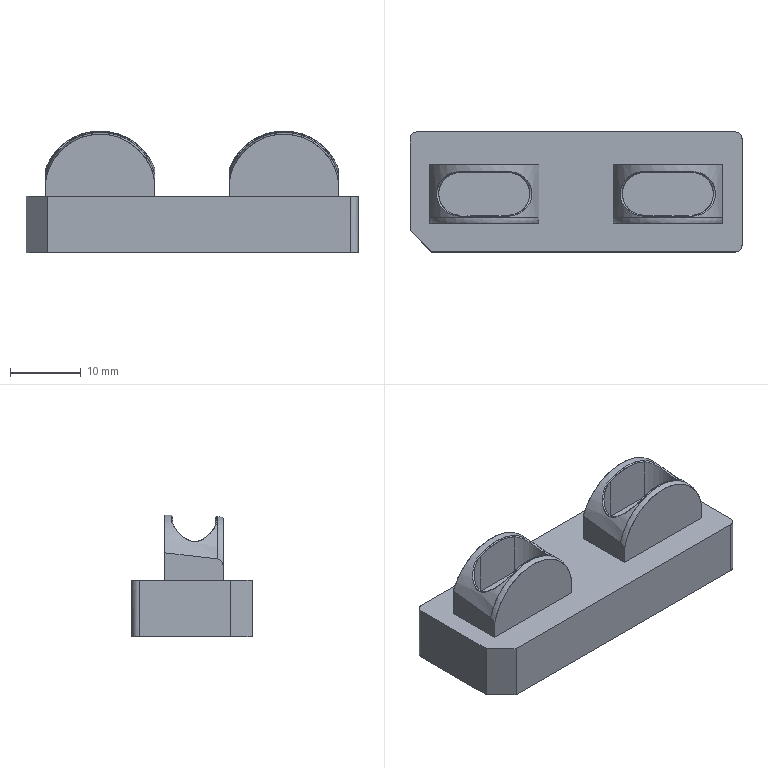NC program | PowerMill | posted with a generic post | part box 47 x 17 x 17.251 mm
Lines 4462 to 5441 of 158620:
N4559 M6
N4560 S18000 M03
N4561 G00 G90 X0.0 Y0.0
N4562 G43 Z9.8013 H15
N4563
N4564 G05 P10000 R4
N4565 X-14.5287 Y6.2823
N4566 Z0.8398
N4567 G01 Z-0.3602 F3000.0
N4568 X-14.5372 Y6.2651 F5000.0
N4569 G03 X-14.4591 Y6.0328 I0.1551 J-0.0771
N4570 G01 X-13.0861 Y5.351
N4571 X-11.3976 Y5.3556
N4572 X-10.9755 Y5.2976
N4573 X-10.5533 Y5.0993
N4574 X-10.2689 Y4.8545
N4575 X-10.1312 Y4.6744
N4576 X-10.0004 Y4.4324
N4577 X-9.8955 Y4.0103
N4578 X-9.9101 Y3.5881
N4579 X-9.989 Y3.166
N4580 X-10.2375 Y2.3217
N4581 X-10.5533 Y1.834
N4582 X-10.9755 Y1.5284
N4583 X-11.0921 Y1.4775
N4584 X-11.3976 Y1.3971
N4585 X-11.8197 Y1.3289
N4586 X-13.0861 Y1.2569
N4587 X-13.9304 Y1.3016
N4588 X-14.3525 Y1.3571
N4589 X-14.9033 Y1.4775
N4590 X-15.1968 Y1.6321
N4591 X-15.5024 Y1.8996
N4592 X-15.6189 Y2.0561
N4593 X-15.7625 Y2.3217
N4594 X-15.9643 Y3.166
N4595 X-15.9654 Y3.1698
N4596 X-16.0893 Y3.5881
N4597 X-16.1065 Y4.0103
N4598 X-15.9967 Y4.4324
N4599 X-15.7305 Y4.8545
N4600 X-15.6189 Y4.9652
N4601 X-15.1968 Y5.2356
N4602 X-14.7747 Y5.3464
N4603 X-13.0861 Y5.351
N4604 G00 Z3.6916
N4605 G01 X-8.4993 Y3.4109 F10000.0
N4606 G00 Z0.6916
N4607 G01 Z-0.5084 F3000.0
N4608 X-8.6872 Y3.4531 F5000.0
N4609 X-9.2876 Y3.5881
N4610 X-9.3825 Y3.166
N4611 X-9.3834 Y3.1593
N4612 Y3.1591
N4613 X-9.4373 Y2.7439
N4614 X-9.5393 Y2.3217
N4615 X-9.7951 Y1.8996
N4616 X-10.1312 Y1.6105
N4617 X-10.3939 Y1.4775
N4618 X-10.9755 Y1.3219
N4619 X-11.3976 Y1.2507
N4620 X-13.0049 Y1.2432
N4621 X-12.9986 Y-0.1067
N4622 X-13.0049 Y1.2432
N4623 X-14.3525 Y1.237
N4624 X-14.7747 Y1.2818
N4625 X-15.1968 Y1.3611
N4626 X-15.6061 Y1.4775
N4627 X-16.0411 Y1.7388
N4628 X-16.2049 Y1.8996
N4629 X-16.4607 Y2.3217
N4630 X-16.5622 Y2.7439
N4631 X-16.614 Y3.166
N4632 X-16.712 Y3.5881
N4633 X-16.729 Y4.0103
N4634 X-16.6181 Y4.4324
N4635 X-16.4632 Y4.7165
N4636 X-16.3566 Y4.8545
N4637 X-16.0411 Y5.1188
N4638 X-15.7173 Y5.2767
N4639 X-15.1968 Y5.3556
N4640 X-10.9755
N4641 X-10.5533 Y5.3396
N4642 X-10.2842 Y5.2767
N4643 X-10.1312 Y5.2159
N4644 X-9.6444 Y4.8545
N4645 X-9.3786 Y4.4324
N4646 X-9.2869 Y4.0958
N4647 X-9.2876 Y3.5881
N4648 X-8.6872 Y3.4531
N4649 G00 Z3.6916
N4650 G01 X-16.0955 Y-2.905 F10000.0
N4651 G00 Z0.6916
N4652 G01 Z-0.5084 F3000.0
N4653 X-15.9152 Y-2.9724 F5000.0
N4654 X-15.3971 Y-3.166
N4655 X-15.2393 Y-2.7439
N4656 X-14.9094 Y-2.3217
N4657 X-14.7747 Y-2.2158
N4658 X-14.3525 Y-2.008
N4659 X-13.9304 Y-1.9389
N4660 X-13.0861 Y-1.8895
N4661 X-11.8197 Y-1.9669
N4662 X-11.3976 Y-2.1073
N4663 X-11.0813 Y-2.3217
N4664 X-10.9755 Y-2.4261
N4665 X-10.7601 Y-2.7439
N4666 X-10.6135 Y-3.166
N4667 X-10.6011 Y-3.5881
N4668 X-10.6794 Y-4.0103
N4669 X-10.8703 Y-4.4324
N4670 X-11.2762 Y-4.8545
N4671 X-11.9014 Y-5.2767
N4672 X-12.2419 Y-5.4019
N4673 X-12.664 Y-5.4604
N4674 X-13.5083 Y-5.448
N4675 X-13.9304 Y-5.3414
N4676 X-14.0974 Y-5.2767
N4677 X-14.3525 Y-5.1351
N4678 X-14.7177 Y-4.8545
N4679 X-15.115 Y-4.4324
N4680 X-15.3071 Y-4.0103
N4681 X-15.4101 Y-3.5881
N4682 X-15.3971 Y-3.166
N4683 X-15.9152 Y-2.9724
N4684 G00 Z3.5434
N4685 G01 X-8.7078 Y5.5542 F10000.0
N4686 G00 Z0.5434
N4687 G01 Z-0.6566 F3000.0
N4688 X-8.8426 Y5.4169 F5000.0
N4689 X-9.2869 Y4.9643
N4690 X-9.1752 Y4.8545
N4691 X-8.9107 Y4.4324
N4692 X-8.8024 Y4.0103
N4693 X-8.8146 Y3.5881
N4694 X-8.9078 Y2.7439
N4695 X-9.0115 Y2.3217
N4696 X-9.2673 Y1.8996
N4697 X-9.7091 Y1.5505
N4698 X-9.8661 Y1.4775
N4699 X-10.5533 Y1.2833
N4700 X-10.9755 Y1.2369
N4701 X-13.0003 Y1.237
N4702 X-13.0018 Y-0.1108
N4703 X-11.1398 Y-0.1129
N4704 G02 X-10.9912 Y-0.2818 I-0.0002 J-0.15
N4705 G01 X-10.9996 Y-0.352
N4706 X-11.007 Y-0.4224
N4707 G02 X-11.1822 Y-0.5555 I-0.1493 J0.0146
N4708 G01 X-11.5872 Y-0.4847
N4709 X-11.6691 Y-0.473
N4710 X-11.7515 Y-0.4663
N4711 X-12.1737 Y-0.4449
N4712 X-12.2077 Y-0.4436
N4713 X-12.2418 Y-0.4432
N4714 X-13.9304 Y-0.4431
N4715 X-14.0297 Y-0.4468
N4716 X-14.1286 Y-0.4578
N4717 X-14.8247 Y-0.5611
N4718 G02 X-14.996 Y-0.427 I-0.022 J0.1484
N4719 G01 X-15.0038 Y-0.3522
N4720 X-15.0126 Y-0.2776
N4721 G02 X-14.8637 Y-0.1088 I0.1488 J0.0188
N4722 G01 X-13.0018 Y-0.1108
N4723 X-13.0003 Y1.237
N4724 X-14.3525
N4725 X-15.1968 Y1.2416
N4726 X-16.0411 Y1.4461
N4727 X-16.4632 Y1.6563
N4728 X-16.7327 Y1.8996
N4729 X-16.8853 Y2.115
N4730 X-16.9884 Y2.3217
N4731 X-17.0903 Y2.7439
N4732 X-17.1855 Y3.5881
N4733 X-17.1974 Y4.0103
N4734 X-17.0892 Y4.4324
N4735 X-16.8244 Y4.8545
N4736 X-16.4632 Y5.1488
N4737 X-16.1857 Y5.2767
N4738 X-16.0411 Y5.3176
N4739 X-15.6189 Y5.3556
N4740 X-10.5533
N4741 X-10.1312 Y5.3465
N4742 X-9.7091 Y5.2362
N4743 X-9.2869 Y4.9643
N4744 X-8.8426 Y5.4169
N4745 G00 Z3.5434
N4746 G01 X-9.1282 Y-2.4659 F10000.0
N4747 G00 Z0.5434
N4748 G01 Z-0.6566 F3000.0
N4749 X-9.3091 Y-2.5319 F5000.0
N4750 X-9.8901 Y-2.7439
N4751 X-9.7361 Y-3.166
N4752 X-9.7208 Y-3.5881
N4753 X-9.7944 Y-4.0103
N4754 X-9.9599 Y-4.4324
N4755 X-10.2246 Y-4.8545
N4756 X-10.5533 Y-5.1515
N4757 X-10.9755 Y-5.4614
N4758 X-11.4883 Y-5.6988
N4759 X-12.2419 Y-5.8911
N4760 X-12.664 Y-5.9219
N4761 X-13.5083 Y-5.9209
N4762 X-13.9304 Y-5.8524
N4763 X-14.3525 Y-5.7518
N4764 X-14.7747 Y-5.5841
N4765 X-15.1968 Y-5.3422
N4766 X-15.6189 Y-5.0146
N4767 X-15.7703 Y-4.8545
N4768 X-16.0411 Y-4.4248
N4769 X-16.2065 Y-4.0103
N4770 X-16.2786 Y-3.5881
N4771 X-16.2567 Y-3.166
N4772 X-16.1135 Y-2.7439
N4773 X-16.0411 Y-2.6265
N4774 X-15.7805 Y-2.3217
N4775 X-15.6189 Y-2.1945
N4776 X-15.1968 Y-2.0001
N4777 X-14.7747 Y-1.9184
N4778 X-13.9304 Y-1.7931
N4779 X-12.2419 Y-1.7932
N4780 X-11.8197 Y-1.8145
N4781 X-10.9755 Y-1.9622
N4782 X-10.5533 Y-2.097
N4783 X-10.1312 Y-2.405
N4784 X-9.8901 Y-2.7439
N4785 X-9.3091 Y-2.5319
N4786 X-7.9132 Y1.8968 Z-0.8048
N4787 X-8.0787 Y1.9953
N4788 X-8.6275 Y2.3217
N4789 X-8.8648 Y1.9228
N4790 X-9.2869 Y1.5717
N4791 X-9.4818 Y1.4775
N4792 X-10.1312 Y1.2644
N4793 X-10.5533 Y1.237
N4794 X-10.9743 Y1.2371
N4795 X-10.9755 Y1.237
N4796 X-13.0053
N4797 X-13.0055 Y-0.1126
N4798 X-10.6693 Y-0.1129
N4799 G02 X-10.5201 Y-0.2789 I0.0 J-0.15
N4800 G01 X-10.5242 Y-0.3179
N4801 X-10.5279 Y-0.357
N4802 G02 X-10.7071 Y-0.4904 I-0.1494 J0.0136
N4803 G01 X-10.8085 Y-0.4738
N4804 X-10.9109 Y-0.465
N4805 X-11.333 Y-0.4448
N4806 X-11.3653 Y-0.4436
N4807 X-11.3976 Y-0.4432
N4808 X-14.7747
N4809 X-14.8692 Y-0.4465
N4810 X-14.9633 Y-0.4564
N4811 X-15.3116 Y-0.5056
N4812 G02 X-15.482 Y-0.3701 I-0.021 J0.1486
N4813 G01 X-15.4862 Y-0.324
N4814 X-15.4909 Y-0.278
N4815 G02 X-15.3417 Y-0.1122 I0.1492 J0.0158
N4816 G01 X-13.0055 Y-0.1126
N4817 X-13.0053 Y1.237
N4818 X-14.3525
N4819 X-14.4757 Y1.2377
N4820 X-15.6189 Y1.2379
N4821 X-16.0411 Y1.3073
N4822 X-16.5183 Y1.4775
N4823 X-16.8853 Y1.6831
N4824 X-17.1168 Y1.8996
N4825 X-17.3075 Y2.183
N4826 X-17.3729 Y2.3217
N4827 X-17.4738 Y2.7439
N4828 X-17.5701 Y3.5881
N4829 X-17.5838 Y4.0103
N4830 X-17.4764 Y4.4324
N4831 X-17.3075 Y4.7306
N4832 X-17.2116 Y4.8545
N4833 X-16.8853 Y5.1274
N4834 X-16.4632 Y5.3085
N4835 X-16.0411 Y5.3556
N4836 X-10.1312
N4837 X-9.7091 Y5.3421
N4838 X-9.4276 Y5.2767
N4839 X-9.2869 Y5.2194
N4840 X-8.8648 Y4.9323
N4841 X-8.7895 Y4.8545
N4842 X-8.5228 Y4.4324
N4843 X-8.4155 Y4.0103
N4844 X-8.5263 Y2.7439
N4845 X-8.6275 Y2.3217
N4846 X-8.0787 Y1.9953
N4847 X-8.5918 Y-2.4747
N4848 X-8.7738 Y-2.5375
N4849 X-9.3719 Y-2.7439
N4850 X-9.2263 Y-3.166
N4851 X-9.1844 Y-3.5881
N4852 X-9.2349 Y-4.0103
N4853 X-9.3938 Y-4.4324
N4854 X-9.6404 Y-4.8545
N4855 X-10.0195 Y-5.2767
N4856 X-10.6174 Y-5.6988
N4857 X-10.9755 Y-5.8538
N4858 X-11.3976 Y-5.9218
N4859 X-12.6027 Y-5.9174
N4860 X-12.664 Y-5.9219
N4861 X-13.5083 Y-5.9209
N4862 X-13.5509 Y-5.9139
N4863 X-13.5625
N4864 X-14.7747 Y-5.9095
N4865 X-15.1968 Y-5.7877
N4866 X-15.3848 Y-5.6988
N4867 X-15.9766 Y-5.2767
N4868 X-16.4632 Y-4.718
N4869 X-16.61 Y-4.4324
N4870 X-16.764 Y-4.0103
N4871 X-16.8142 Y-3.5881
N4872 X-16.7754 Y-3.166
N4873 X-16.6269 Y-2.7439
N4874 X-16.4632 Y-2.4982
N4875 X-16.2953 Y-2.3217
N4876 X-16.0411 Y-2.1405
N4877 X-15.6189 Y-1.9745
N4878 X-15.1968 Y-1.8528
N4879 X-14.7747 Y-1.7932
N4880 X-13.9305
N4881 X-13.9304
N4882 X-13.0137
N4883 X-11.3976
N4884 X-10.9755 Y-1.8134
N4885 X-10.1312 Y-2.057
N4886 X-9.7061 Y-2.3217
N4887 X-9.3719 Y-2.7439
N4888 X-8.7738 Y-2.5375
N4889 G00 Z3.2471
N4890 G01 X-7.7299 Y5.2969 F10000.0
N4891 G00 Z0.2471
N4892 G01 Z-0.953 F3000.0
N4893 X-7.8931 Y5.1948 F5000.0
N4894 X-8.4364 Y4.8545
N4895 X-8.1721 Y4.4324
N4896 X-8.0634 Y4.0103
N4897 X-8.0792 Y3.5881
N4898 X-8.1588 Y2.7439
N4899 X-8.2605 Y2.3217
N4900 X-8.5164 Y1.8996
N4901 X-8.8648 Y1.6017
N4902 X-9.1144 Y1.4775
N4903 X-9.7091 Y1.2733
N4904 X-10.1312 Y1.2369
N4905 X-10.5533 Y1.2371
N4906 X-10.9743 Y1.2372
N4907 X-10.9755 Y1.237
N4908 X-12.9966 Y1.2371
N4909 X-12.9971 Y-0.112
N4910 X-10.2318 Y-0.113
N4911 G02 X-10.0825 Y-0.2766 I-0.0001 J-0.15
N4912 G01 X-10.0855 Y-0.3113
N4913 X-10.0883 Y-0.346
N4914 G02 X-10.2694 Y-0.4811 I-0.1496 J0.0115
N4915 G01 X-10.4095 Y-0.4586
N4916 X-10.5511 Y-0.4509
N4917 X-15.1945 Y-0.4431
N4918 X-15.2511 Y-0.4442
N4919 X-15.3077 Y-0.4477
N4920 X-15.7298 Y-0.4825
N4921 X-15.7361 Y-0.483
N4922 X-15.7425 Y-0.4836
N4923 G02 X-15.9058 Y-0.346 I-0.0137 J0.1494
N4924 G01 X-15.9087 Y-0.3104
N4925 X-15.9119 Y-0.2748
N4926 G02 X-15.7625 Y-0.1109 I0.1494 J0.0139
N4927 G01 X-12.9971 Y-0.112
N4928 X-12.9966 Y1.2371
N4929 X-14.3525
N4930 X-14.4757 Y1.2377
N4931 X-15.6189 Y1.2379
N4932 X-15.628 Y1.2388
N4933 X-15.6371 Y1.2391
N4934 X-16.0411 Y1.2392
N4935 X-16.4632 Y1.3219
N4936 X-16.8859 Y1.4775
N4937 X-17.3075 Y1.7277
N4938 X-17.4841 Y1.8996
N4939 X-17.7296 Y2.2983
N4940 X-17.8415 Y2.7439
N4941 X-17.8906 Y3.166
N4942 X-17.9362 Y4.0103
N4943 X-17.8292 Y4.4324
N4944 X-17.7296 Y4.6267
N4945 X-17.5636 Y4.8545
N4946 X-17.3075 Y5.0817
N4947 X-16.9249 Y5.2767
N4948 X-16.4632 Y5.3555
N4949 X-16.042
N4950 X-16.0411 Y5.3556
N4951 X-11.6923
N4952 X-9.7091
N4953 X-9.2869 Y5.3312
N4954 X-9.0769 Y5.2767
N4955 X-8.8648 Y5.1867
N4956 X-8.4364 Y4.8545
N4957 X-7.8931 Y5.1948
N4958 G00 Z3.2471
N4959 G01 X-17.1424 Y-5.793 F10000.0
N4960 G00 Z0.2471
N4961 G01 Z-0.953 F3000.0
N4962 X-16.9917 Y-5.6732 F5000.0
N4963 X-16.4927 Y-5.2767
N4964 X-16.8281 Y-4.8545
N4965 X-17.0647 Y-4.4324
N4966 X-17.2103 Y-4.0103
N4967 X-17.2635 Y-3.5881
N4968 X-17.2355 Y-3.166
N4969 X-17.0912 Y-2.7439
N4970 X-16.8853 Y-2.4479
N4971 X-16.7602 Y-2.3217
N4972 X-16.4632 Y-2.118
N4973 X-16.0411 Y-1.9489
N4974 X-15.6189 Y-1.8279
N4975 X-15.1968 Y-1.7931
N4976 X-10.9755 Y-1.7932
N4977 X-10.5533 Y-1.8009
N4978 X-10.1285 Y-1.8996
N4979 X-9.7091 Y-2.0388
N4980 X-9.2869 Y-2.283
N4981 X-8.9087 Y-2.7439
N4982 X-8.7613 Y-3.166
N4983 X-8.7355 Y-3.5881
N4984 X-8.7912 Y-4.0103
N4985 X-8.9353 Y-4.4324
N4986 X-9.2869 Y-5.0256
N4987 X-9.5048 Y-5.2767
N4988 X-9.7091 Y-5.4619
N4989 X-10.0333 Y-5.6988
N4990 X-10.1312 Y-5.755
N4991 X-10.5533 Y-5.8981
N4992 X-10.9755 Y-5.9219
N4993 X-15.1968
N4994 X-15.6189 Y-5.8563
N4995 X-15.9684 Y-5.6988
N4996 X-16.4927 Y-5.2767
N4997 X-16.9917 Y-5.6732
N4998 G00 Z3.0989
N4999 G01 X-7.1779 Y1.9584 F10000.0
N5000 G00 Z0.0989
N5001 G01 Z-1.1011 F3000.0
N5002 X-7.3513 Y2.042 F5000.0
N5003 X-7.9316 Y2.3217
N5004 X-8.0205 Y2.1372
N5005 X-8.1803 Y1.8996
N5006 X-8.4427 Y1.6545
N5007 X-8.754 Y1.4775
N5008 X-9.2869 Y1.2872
N5009 X-9.7091 Y1.237
N5010 X-10.131
N5011 X-10.1312
N5012 X-10.178
N5013 X-13.002
N5014 X-13.0033 Y-0.1098
N5015 X-9.8888 Y-0.1128
N5016 G02 X-9.7395 Y-0.2758 I-0.0001 J-0.15
N5017 G01 X-9.7417 Y-0.3021
N5018 X-9.7438 Y-0.3285
N5019 G02 X-9.9171 Y-0.4652 I-0.1495 J0.0114
N5020 G01 X-10.0232 Y-0.4525
N5021 X-10.13 Y-0.4481
N5022 X-15.6177 Y-0.4431
N5023 X-15.6625 Y-0.4438
N5024 X-15.7072 Y-0.446
N5025 X-16.1028 Y-0.4719
N5026 G02 X-16.2621 Y-0.3338 I-0.0098 J0.1497
N5027 G01 X-16.2647 Y-0.302
N5028 X-16.2674 Y-0.2702
N5029 G02 X-16.1179 Y-0.1068 I0.1494 J0.0134
N5030 G01 X-13.0033 Y-0.1098
N5031 X-13.002 Y1.237
N5032 X-16.0411 Y1.2369
N5033 X-16.4632 Y1.2435
N5034 X-16.8853 Y1.3439
N5035 X-17.2455 Y1.4775
N5036 X-17.7296 Y1.8025
N5037 X-17.8199 Y1.8996
N5038 X-18.0711 Y2.3217
N5039 X-18.1517 Y2.6117
N5040 X-18.2371 Y4.0103
N5041 X-18.1517 Y4.3717
N5042 X-17.8642 Y4.8545
N5043 X-17.7296 Y4.9854
N5044 X-17.3075 Y5.2448
N5045 X-16.8853 Y5.3478
N5046 X-16.4632 Y5.3556
N5047 X-9.2869
N5048 X-8.8648 Y5.303
N5049 X-8.4427 Y5.1158
N5050 X-8.1359 Y4.8545
N5051 X-8.0205 Y4.705
N5052 X-7.8704 Y4.4324
N5053 X-7.763 Y4.0103
N5054 X-7.8365 Y2.7439
N5055 X-7.9316 Y2.3217
N5056 X-7.3513 Y2.042
N5057 X-7.7599 Y-2.467
N5058 X-7.9416 Y-2.5305
N5059 X-8.553 Y-2.7439
N5060 X-8.4057 Y-3.166
N5061 X-8.3742 Y-3.5881
N5062 X-8.4237 Y-4.0103
N5063 X-8.5362 Y-4.4324
N5064 X-8.8648 Y-5.0118
N5065 X-9.2869 Y-5.4692
N5066 X-9.5728 Y-5.6988
N5067 X-9.7091 Y-5.7727
N5068 X-10.1312 Y-5.9042
N5069 X-10.5533 Y-5.9219
N5070 X-15.6189
N5071 X-16.0411 Y-5.8671
N5072 X-16.4264 Y-5.6988
N5073 X-16.9044 Y-5.2767
N5074 X-17.2394 Y-4.8545
N5075 X-17.4634 Y-4.4324
N5076 X-17.5746 Y-4.0103
N5077 X-17.6261 Y-3.5881
N5078 X-17.5927 Y-3.166
N5079 X-17.4464 Y-2.7439
N5080 X-17.3075 Y-2.5282
N5081 X-17.1158 Y-2.3217
N5082 X-16.8853 Y-2.1559
N5083 X-16.4632 Y-1.9648
N5084 X-16.0411 Y-1.8208
N5085 X-15.6189 Y-1.7931
N5086 X-10.5533 Y-1.7932
N5087 X-10.1312 Y-1.7981
N5088 X-9.7091 Y-1.8923
N5089 X-9.2869 Y-2.0662
N5090 X-8.8844 Y-2.3217
N5091 X-8.553 Y-2.7439
N5092 X-7.9416 Y-2.5305
N5093 G00 Z2.9507
N5094 G01 X-7.4348 Y5.6198 F10000.0
N5095 G00 Z-0.0493
N5096 G01 Z-1.2493 F3000.0
N5097 X-7.5682 Y5.4811 F5000.0
N5098 X-8.0205 Y5.0109
N5099 X-7.858 Y4.8545
N5100 X-7.5927 Y4.4324
N5101 X-7.4866 Y4.0103
N5102 X-7.4934 Y3.5881
N5103 X-7.5428 Y3.166
N5104 X-7.5522 Y2.7439
N5105 X-7.6377 Y2.3217
N5106 X-7.8722 Y1.8996
N5107 X-8.0205 Y1.7385
N5108 X-8.3986 Y1.4775
N5109 X-8.8648 Y1.314
N5110 X-9.2869 Y1.2301
N5111 X-11.1423 Y1.2353
N5112 X-12.9977 Y1.238
N5113 X-13.0009 Y-0.1109
N5114 X-9.549 Y-0.1192
N5115 G02 X-9.3998 Y-0.2813 I-0.0004 J-0.15
N5116 G01 X-9.4015 Y-0.3028
N5117 X-9.4031 Y-0.3242
N5118 G02 X-9.5684 Y-0.4627 I-0.1496 J0.0107
N5119 G01 X-9.6192 Y-0.4583
N5120 X-9.6702 Y-0.4559
N5121 X-10.0923 Y-0.4437
N5122 X-10.1117 Y-0.4433
N5123 X-10.1312 Y-0.4431
N5124 X-16.0411
N5125 X-16.1107 Y-0.4449
N5126 X-16.1801 Y-0.4503
N5127 X-16.432 Y-0.4764
N5128 G02 X-16.5971 Y-0.3376 I-0.0155 J0.1492
N5129 G01 X-16.5998 Y-0.3013
N5130 X-16.6027 Y-0.2651
N5131 G02 X-16.4528 Y-0.1025 I0.1495 J0.0126
N5132 G01 X-13.0009 Y-0.1109
N5133 X-12.9977 Y1.238
N5134 X-14.5194 Y1.2383
N5135 X-16.0411 Y1.237
N5136 X-16.4632 Y1.2436
N5137 X-16.4799 Y1.2475
N5138 X-16.4969 Y1.2476
N5139 X-16.8853 Y1.2485
N5140 X-17.6016 Y1.4775
N5141 X-17.7296 Y1.5477
N5142 X-18.1294 Y1.8996
N5143 X-18.3644 Y2.3217
N5144 X-18.4508 Y2.7439
N5145 X-18.5141 Y4.0103
N5146 X-18.4074 Y4.4324
N5147 X-18.1415 Y4.8545
N5148 X-17.7296 Y5.1787
N5149 X-17.5033 Y5.2767
N5150 X-17.3075 Y5.3281
N5151 X-16.8853 Y5.3556
N5152 X-9.2869
N5153 X-8.8648 Y5.351
N5154 X-8.4973 Y5.2767
N5155 X-8.0205 Y5.0109
N5156 X-7.5682 Y5.4811
N5157 G00 Z2.9507
N5158 G01 X-7.4038 Y-2.4666 F10000.0
N5159 G00 Z-0.0493
N5160 G01 Z-1.2493 F3000.0
N5161 X-7.5855 Y-2.5301 F5000.0
N5162 X-8.1975 Y-2.7439
N5163 X-8.05 Y-3.166
N5164 X-8.031 Y-3.5881
N5165 X-8.0904 Y-4.0103
N5166 X-8.2147 Y-4.4324
N5167 X-8.4427 Y-4.8799
N5168 X-8.8648 Y-5.4243
N5169 X-9.1933 Y-5.6988
N5170 X-9.7091 Y-5.8967
N5171 X-10.1312 Y-5.9219
N5172 X-12.4171
N5173 X-15.6189
N5174 X-15.6195 Y-5.9218
N5175 X-15.6235
N5176 X-16.0411
N5177 X-16.4632 Y-5.8536
N5178 X-16.8058 Y-5.6988
N5179 X-17.2593 Y-5.2767
N5180 X-17.5709 Y-4.8545
N5181 X-17.7296 Y-4.558
N5182 X-17.9096 Y-4.0103
N5183 X-17.9693 Y-3.5881
N5184 X-17.9498 Y-3.166
N5185 X-17.8015 Y-2.7439
N5186 X-17.7296 Y-2.6217
N5187 X-17.4715 Y-2.3217
N5188 X-17.3075 Y-2.1954
N5189 X-16.8853 Y-1.9923
N5190 X-16.4632 Y-1.8368
N5191 X-16.0411 Y-1.7931
N5192 X-10.1312
N5193 X-9.7091 Y-1.8053
N5194 X-9.2869 Y-1.9225
N5195 X-8.8648 Y-2.0979
N5196 X-8.5289 Y-2.3217
N5197 X-8.4427 Y-2.4053
N5198 X-8.1975 Y-2.7439
N5199 X-7.5855 Y-2.5301
N5200 G00 Z2.8025
N5201 G01 X-19.1493 Y1.4818 F10000.0
N5202 G00 Z-0.1975
N5203 G01 Z-1.3975 F3000.0
N5204 X-18.9823 Y1.5775 F5000.0
N5205 X-18.4201 Y1.8996
N5206 X-18.5739 Y2.168
N5207 X-18.633 Y2.3217
N5208 X-18.7064 Y2.7439
N5209 X-18.7743 Y4.0103
N5210 X-18.6653 Y4.4324
N5211 X-18.5739 Y4.616
N5212 X-18.3991 Y4.8545
N5213 X-18.1517 Y5.0775
N5214 X-17.7605 Y5.2767
N5215 X-17.3075 Y5.3554
N5216 X-16.8883
N5217 X-16.8853 Y5.3556
N5218 X-10.3954
N5219 X-8.8648
N5220 X-8.4427 Y5.3301
N5221 X-8.2395 Y5.2767
N5222 X-8.0205 Y5.1835
N5223 X-7.5984 Y4.8528
N5224 X-7.333 Y4.4324
N5225 X-7.2279 Y4.0103
N5226 X-7.2933 Y2.7439
N5227 X-7.3629 Y2.3217
N5228 X-7.5757 Y1.8996
N5229 X-8.0459 Y1.4775
N5230 X-8.4427 Y1.3207
N5231 X-8.8648 Y1.2161
N5232 X-9.2869 Y1.209
N5233 X-9.6184 Y1.231
N5234 X-13.0443 Y1.238
N5235 X-16.4703 Y1.2381
N5236 X-16.8853 Y1.1979
N5237 X-17.3075 Y1.2546
N5238 X-17.7296 Y1.3717
N5239 X-17.9533 Y1.4775
N5240 X-18.1517 Y1.6144
N5241 X-18.4201 Y1.8996
N5242 X-18.9823 Y1.5775
N5243 G00 Z2.8025
N5244 G01 X-7.0979 Y-2.4795 F10000.0
N5245 G00 Z-0.1975
N5246 G01 Z-1.3975 F3000.0
N5247 X-7.2807 Y-2.5398 F5000.0
N5248 X-7.8993 Y-2.7439
N5249 X-7.76 Y-3.166
N5250 X-7.7468 Y-3.5881
N5251 X-7.797 Y-4.0103
N5252 X-7.9053 Y-4.4324
N5253 X-8.106 Y-4.8545
N5254 X-8.4161 Y-5.2767
N5255 X-8.8713 Y-5.6988
N5256 X-9.2869 Y-5.8749
N5257 X-9.7091 Y-5.9219
N5258 X-16.0411
N5259 X-16.4632 Y-5.9152
N5260 X-16.8853 Y-5.8195
N5261 X-17.129 Y-5.6988
N5262 X-17.3075 Y-5.5676
N5263 X-17.7296 Y-5.1015
N5264 X-17.8934 Y-4.8545
N5265 X-18.0947 Y-4.4324
N5266 X-18.1517 Y-4.2443
N5267 X-18.2556 Y-3.5881
N5268 X-18.24 Y-3.166
N5269 X-18.1008 Y-2.7439
N5270 X-17.7831 Y-2.3217
N5271 X-17.3075 Y-2.022
N5272 X-16.8853 Y-1.8578
N5273 X-16.4632 Y-1.7926
N5274 X-13.0861 Y-1.7929
N5275 X-13.086 Y-0.4429
N5276 X-16.4631 Y-0.4426
N5277 X-16.5665 Y-0.4466
N5278 X-16.6693 Y-0.4584
N5279 X-16.7229 Y-0.4667
N5280 G02 X-16.8954 Y-0.3289 I-0.0229 J0.1482
N5281 G01 X-16.8962 Y-0.3178
N5282 X-16.897 Y-0.3068
N5283 G02 X-16.7615 Y-0.1464 I0.1496 J0.0111
N5284 G01 X-16.7552 Y-0.1458
N5285 X-16.4131 Y-0.1127
N5286 X-16.4058 Y-0.1122
N5287 X-16.3985 Y-0.112
N5288 X-9.6687 Y-0.119
N5289 X-9.6638
N5290 X-9.6589 Y-0.1193
N5291 X-9.3762 Y-0.138
N5292 X-9.3202 Y-0.1406
N5293 X-9.2642 Y-0.1408
N5294 X-9.2539 Y-0.1406
N5295 G02 X-9.1018 Y-0.3018 I0.0026 J-0.15
N5296 G01 X-9.1027 Y-0.3139
N5297 X-9.1035 Y-0.3259
N5298 G02 X-9.2612 Y-0.4652 I-0.1497 J0.0105
N5299 G01 X-9.6368 Y-0.4451
N5300 X-9.6729 Y-0.4436
N5301 X-9.709 Y-0.4431
N5302 X-13.086 Y-0.4429
N5303 X-13.0861 Y-1.7929
N5304 X-9.7091 Y-1.7931
N5305 X-9.2869 Y-1.8158
N5306 X-8.9947 Y-1.8996
N5307 X-8.4427 Y-2.1491
N5308 X-8.2166 Y-2.3217
N5309 X-8.0205 Y-2.5473
N5310 X-7.8993 Y-2.7439
N5311 X-7.2807 Y-2.5398
N5312 G00 Z2.6543
N5313 G01 X-6.4197 Y4.9445 F10000.0
N5314 G00 Z-0.3457
N5315 G01 Z-1.5457 F3000.0
N5316 X-6.5922 Y4.8591 F5000.0
N5317 X-7.1763 Y4.5699
N5318 X-7.1082 Y4.4324
N5319 X-7.0011 Y4.0103
N5320 X-7.026 Y3.166
N5321 X-7.112 Y2.3217
N5322 X-7.1763 Y2.133
N5323 X-7.2998 Y1.8996
N5324 X-7.5984 Y1.5583
N5325 X-7.7046 Y1.4775
N5326 X-8.0205 Y1.3101
N5327 X-8.4427 Y1.206
N5328 X-8.8648 Y1.1497
N5329 X-9.6523 Y1.2311
N5330 X-13.0577 Y1.2381
N5331 X-16.4632 Y1.2378
N5332 X-16.8853 Y1.1683
N5333 X-17.3075 Y1.1564
N5334 X-17.7296 Y1.2409
N5335 X-18.1517 Y1.3927
N5336 X-18.2925 Y1.4775
N5337 X-18.5739 Y1.7281
N5338 X-18.7023 Y1.8996
N5339 X-18.89 Y2.3217
N5340 X-18.9464 Y2.7439
N5341 X-19.0012 Y4.0103
N5342 X-18.8914 Y4.4324
N5343 X-18.6259 Y4.8545
N5344 X-18.1517 Y5.209
N5345 X-17.9869 Y5.2767
N5346 X-17.7296 Y5.3384
N5347 X-17.3076 Y5.3556
N5348 X-16.8853 Y5.3555
N5349 X-10.3954
N5350 X-8.8648 Y5.3556
N5351 X-8.8403 Y5.3541
N5352 X-8.8359
N5353 X-8.4427 Y5.354
N5354 X-8.0129 Y5.2767
N5355 X-7.5984 Y5.0585
N5356 X-7.3739 Y4.8545
N5357 X-7.1763 Y4.5699
N5358 X-6.5922 Y4.8591
N5359 G00 Z2.8128
N5360 G01 X-19.3007 Y-4.1307 F10000.0
N5361 G00 Z-0.3457
N5362 G01 Z-1.5457 F3000.0
N5363 X-19.1102 Y-4.1033 F5000.0
N5364 X-18.465 Y-4.0103
N5365 X-18.5259 Y-3.5881
N5366 X-18.5195 Y-3.166
N5367 X-18.3913 Y-2.7439
N5368 X-18.1517 Y-2.3851
N5369 X-17.7296 Y-2.0588
N5370 X-17.3195 Y-1.8996
N5371 X-16.8853 Y-1.7866
N5372 X-16.0959 Y-1.7927
N5373 X-13.116 Y-1.7929
N5374 X-13.1147 Y-0.44
N5375 X-16.4914 Y-0.437
N5376 G02 X-16.5156 Y-0.139 I0.0001 J0.15
N5377 G01 X-16.3657 Y-0.1143
N5378 X-16.3535 Y-0.1128
N5379 X-16.3412 Y-0.1123
N5380 X-9.7302 Y-0.1188
N5381 X-9.7225 Y-0.119
N5382 X-9.7149 Y-0.1196
N5383 X-9.5467 Y-0.137
N5384 G02 X-9.5563 Y-0.4361 I-0.0155 J-0.1492
N5385 G01 X-9.732 Y-0.443
N5386 X-9.735 Y-0.4431
N5387 X-9.738
N5388 X-13.1147 Y-0.44
N5389 X-13.116 Y-1.7929
N5390 X-10.4314 Y-1.7931
N5391 X-9.7091
N5392 X-9.2869 Y-1.7765
N5393 X-8.8648 Y-1.8357
N5394 X-8.4427 Y-1.9821
N5395 X-8.0205 Y-2.2229
N5396 X-7.9094 Y-2.3217
N5397 X-7.6094 Y-2.7439
N5398 X-7.4813 Y-3.166
N5399 X-7.4759 Y-3.5881
N5400 X-7.5331 Y-4.0103
N5401 X-7.5984 Y-4.2846
N5402 X-7.8368 Y-4.8545
N5403 X-8.1218 Y-5.2767
N5404 X-8.4427 Y-5.611
N5405 X-8.5676 Y-5.6988
N5406 X-8.8648 Y-5.8394
N5407 X-9.2869 Y-5.9194
N5408 X-9.6877 Y-5.9195
N5409 X-9.6958 Y-5.9204
N5410 X-9.7091 Y-5.9219
N5411 X-16.0411
N5412 X-16.4634
N5413 X-16.8853 Y-5.9019
N5414 X-17.3075 Y-5.7662
N5415 X-17.4323 Y-5.6988
N5416 X-17.7296 Y-5.4557
N5417 X-18.1517 Y-4.8773
N5418 X-18.3546 Y-4.4324
N5419 X-18.465 Y-4.0103
N5420 X-19.1102 Y-4.1033
N5421 G00 Z2.667
N5422 G01 X-6.3399 Y1.4254 F10000.0
N5423 G00 Z-0.4939
N5424 G01 Z-1.6939 F3000.0
N5425 X-6.4988 Y1.534 F5000.0
N5426 X-7.0334 Y1.8996
N5427 X-7.1763 Y1.6906
N5428 X-7.3878 Y1.4775
N5429 X-7.5984 Y1.3352
N5430 X-8.0205 Y1.1723
N5431 X-8.4427 Y1.0996
N5432 X-8.8648 Y1.1019
N5433 X-9.2174 Y1.1862
N5434 X-9.6523 Y1.2312
N5435 X-9.6597
N5436 X-13.0614 Y1.2382
N5437 X-16.4632 Y1.2369
N5438 X-17.3075 Y1.0866
N5439 X-17.7296 Y1.1291
N5440 X-18.1517 Y1.2165
N5441 X-18.5739 Y1.4428
N5442 X-18.9684 Y1.8996
N5443 X-19.1277 Y2.3217
N5444 X-19.1669 Y2.7439
N5445 X-19.2192 Y4.0103
N5446 X-19.1111 Y4.4324
N5447 X-18.996 Y4.6504
N5448 X-18.8453 Y4.8545
N5449 X-18.5739 Y5.0926
N5450 X-18.2066 Y5.2767
N5451 X-17.7296 Y5.3556
N5452 X-8.4427
N5453 X-8.0205 Y5.3326
N5454 X-7.7939 Y5.2767
N5455 X-7.5984 Y5.1945
N5456 X-7.1763 Y4.878
N5457 X-6.8899 Y4.4324
N5458 X-6.7821 Y4.0103
N5459 X-6.7912 Y3.5881
N5460 X-6.873 Y2.3217
N5461 X-7.0334 Y1.8996
N5462 X-6.4988 Y1.534
N5463 G00 Z2.667
N5464 G01 X-18.8405 Y-5.7507 F10000.0
N5465 G00 Z-0.4939
N5466 G01 Z-1.6939 F3000.0
N5467 X-18.6809 Y-5.643 F5000.0
N5468 X-18.1379 Y-5.2767
N5469 X-18.4226 Y-4.8545
N5470 X-18.6144 Y-4.4324
N5471 X-18.719 Y-4.0103
N5472 X-18.765 Y-3.5881
N5473 X-18.772 Y-3.166
N5474 X-18.6608 Y-2.7439
N5475 X-18.5739 Y-2.5729
N5476 X-18.3882 Y-2.3217
N5477 X-18.1517 Y-2.1133
N5478 X-17.7296 Y-1.9033
N5479 X-17.3075 Y-1.7789
N5480 X-16.8853 Y-1.7447
N5481 X-16.4674 Y-1.7899
N5482 X-16.4601
N5483 X-16.4046 Y-1.7904
N5484 X-13.0642 Y-1.7917
N5485 X-13.0636 Y-0.4415
N5486 X-16.3803 Y-0.44
N5487 X-16.3882 Y-0.4398
N5488 X-16.3961 Y-0.4391
N5489 X-16.4594 Y-0.4324
N5490 G02 X-16.4699 Y-0.1356 I0.0158 J0.1492
N5491 G01 X-16.3576 Y-0.1156
N5492 X-16.3445 Y-0.1138
N5493 X-16.3312 Y-0.1133
N5494 X-9.7362 Y-0.1187
N5495 X-9.7287 Y-0.1189
N5496 X-9.7212 Y-0.1195
N5497 X-9.5649 Y-0.1354
N5498 G02 X-9.5725 Y-0.4344 I-0.0152 J-0.1492
N5499 G01 X-9.7392 Y-0.4429
N5500 X-9.7431 Y-0.4431
N5501 X-9.7469
N5502 X-13.0636 Y-0.4415
N5503 X-13.0642 Y-1.7917
N5504 X-9.7091 Y-1.7931
N5505 X-8.8648 Y-1.7502
N5506 X-8.4427 Y-1.8528
N5507 X-8.0205 Y-2.0073
N5508 X-7.6116 Y-2.3217
N5509 X-7.3386 Y-2.7439
N5510 X-7.2272 Y-3.166
N5511 X-7.2354 Y-3.5881
N5512 X-7.2803 Y-4.0103
N5513 X-7.386 Y-4.4324
N5514 X-7.5984 Y-4.8943
N5515 X-8.0205 Y-5.4668
N5516 X-8.3077 Y-5.6988
N5517 X-8.4427 Y-5.7717
N5518 X-8.8648 Y-5.9035
N5519 X-9.2869 Y-5.9219
N5520 X-16.8853
N5521 X-17.3075 Y-5.8658
N5522 X-17.6922 Y-5.6988
N5523 X-18.1379 Y-5.2767
N5524 X-18.6809 Y-5.643
N5525 G00 Z2.8474
N5526 G01 X-6.6153 Y5.6906 F10000.0
N5527 G00 Z-0.6421
N5528 G01 Z-1.8421 F3000.0
N5529 X-6.744 Y5.5475 F5000.0
N5530 X-7.1763 Y5.0671
N5531 X-6.94 Y4.8545
N5532 X-6.7541 Y4.5932
N5533 X-6.6748 Y4.4324
N5534 X-6.5674 Y4.0103
N5535 X-6.5724 Y3.5881
N5536 X-6.6537 Y2.3217
N5537 X-6.7541 Y1.9701
N5538 X-7.0875 Y1.4775